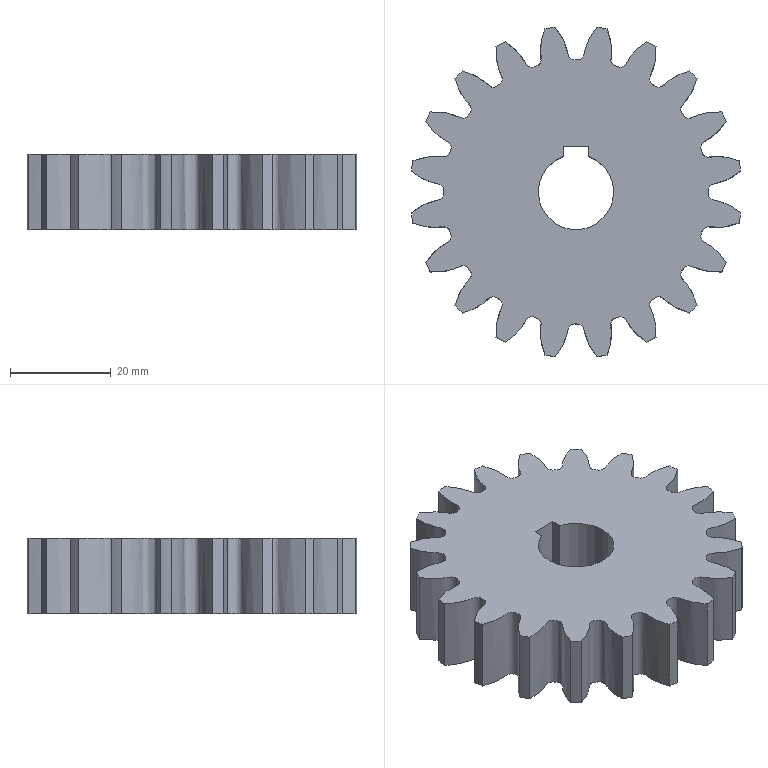Part | STEP file | Cuon T phu H01_5_Spur01 | 1 solid | 48 faces | box 65.481 x 65.481 x 15 mm | volume 39369 mm3 | cylinder 23 | spline 20 | plane 5 | commonest cylinder face diameters 66 x20 15 x3